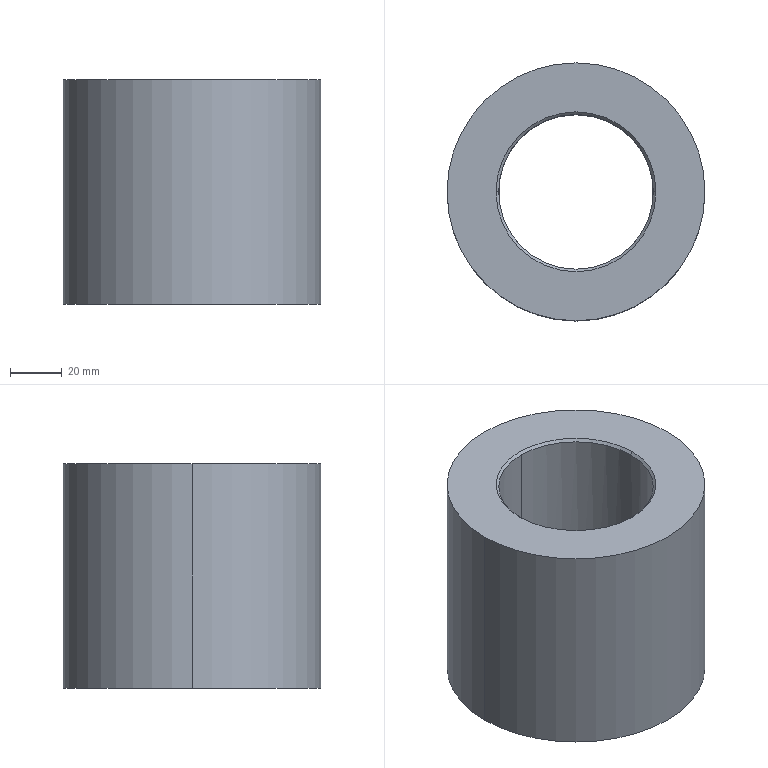Part | SolidWorks | features BaseBody 1 | 1 solid | 8 faces | box 100 x 100 x 87 mm | volume 437214 mm3 | cylinder 4 | cone 2 | plane 2 | commonest cylinder face diameters 60 x2 100 x2
STEP:
#1=CARTESIAN_POINT('',(-30.,0.,41.));
#2=VERTEX_POINT('',#1);
#3=CARTESIAN_POINT('',(0.,-30.,41.));
#4=VERTEX_POINT('',#3);
#5=CARTESIAN_POINT('',(0.,0.,41.));
#6=DIRECTION('',(0.,0.,1.));
#7=DIRECTION('',(-1.,0.,0.));
#8=AXIS2_PLACEMENT_3D('',#5,#6,#7);
#9=CIRCLE('',#8,30.);
#10=EDGE_CURVE('',#2,#4,#9,.T.);
#11=ORIENTED_EDGE('',*,*,#10,.F.);
#12=CARTESIAN_POINT('',(-31.,0.,42.));
#13=VERTEX_POINT('',#12);
#14=CARTESIAN_POINT('',(-31.,0.,42.));
#15=DIRECTION('',(-0.7071,0.,0.7071));
#16=VECTOR('',#15,1000.);
#17=LINE('',#14,#16);
#18=EDGE_CURVE('',#2,#13,#17,.T.);
#19=ORIENTED_EDGE('',*,*,#18,.T.);
#20=CARTESIAN_POINT('',(31.,0.,42.));
#21=VERTEX_POINT('',#20);
#22=CARTESIAN_POINT('',(0.,0.,42.));
#23=DIRECTION('',(0.,0.,-1.));
#24=DIRECTION('',(-1.,0.,0.));
#25=AXIS2_PLACEMENT_3D('',#22,#23,#24);
#26=CIRCLE('',#25,31.);
#27=EDGE_CURVE('',#21,#13,#26,.T.);
#28=ORIENTED_EDGE('',*,*,#27,.F.);
#29=CARTESIAN_POINT('',(30.,0.,41.));
#30=VERTEX_POINT('',#29);
#31=CARTESIAN_POINT('',(31.,0.,42.));
#32=DIRECTION('',(0.7071,0.,0.7071));
#33=VECTOR('',#32,1000.);
#34=LINE('',#31,#33);
#35=EDGE_CURVE('',#30,#21,#34,.T.);
#36=ORIENTED_EDGE('',*,*,#35,.F.);
#37=CARTESIAN_POINT('',(0.,0.,41.));
#38=DIRECTION('',(0.,0.,1.));
#39=DIRECTION('',(-1.,0.,0.));
#40=AXIS2_PLACEMENT_3D('',#37,#38,#39);
#41=CIRCLE('',#40,30.);
#42=EDGE_CURVE('',#4,#30,#41,.T.);
#43=ORIENTED_EDGE('',*,*,#42,.F.);
#44=EDGE_LOOP('',(#11,#19,#28,#36,#43));
#45=FACE_OUTER_BOUND('',#44,.T.);
#46=CARTESIAN_POINT('',(0.,0.,42.));
#47=DIRECTION('',(0.,0.,1.));
#48=DIRECTION('',(1.,0.,0.));
#49=AXIS2_PLACEMENT_3D('',#46,#47,#48);
#50=CONICAL_SURFACE('',#49,31.,0.7854);
#51=ADVANCED_FACE('',(#45),#50,.F.);
#52=ORIENTED_EDGE('',*,*,#42,.T.);
#53=CARTESIAN_POINT('',(0.,30.,41.));
#54=VERTEX_POINT('',#53);
#55=CARTESIAN_POINT('',(0.,0.,41.));
#56=DIRECTION('',(0.,0.,1.));
#57=DIRECTION('',(-1.,0.,0.));
#58=AXIS2_PLACEMENT_3D('',#55,#56,#57);
#59=CIRCLE('',#58,30.);
#60=EDGE_CURVE('',#30,#54,#59,.T.);
#61=ORIENTED_EDGE('',*,*,#60,.T.);
#62=CARTESIAN_POINT('',(0.,30.,-45.));
#63=VERTEX_POINT('',#62);
#64=CARTESIAN_POINT('',(0.,30.,47.));
#65=DIRECTION('',(0.,0.,-1.));
#66=VECTOR('',#65,1000.);
#67=LINE('',#64,#66);
#68=EDGE_CURVE('',#54,#63,#67,.T.);
#69=ORIENTED_EDGE('',*,*,#68,.T.);
#70=CARTESIAN_POINT('',(0.,-30.,-45.));
#71=VERTEX_POINT('',#70);
#72=CARTESIAN_POINT('',(0.,0.,-45.));
#73=DIRECTION('',(0.,0.,1.));
#74=DIRECTION('',(1.,0.,0.));
#75=AXIS2_PLACEMENT_3D('',#72,#73,#74);
#76=CIRCLE('',#75,30.);
#77=EDGE_CURVE('',#71,#63,#76,.T.);
#78=ORIENTED_EDGE('',*,*,#77,.F.);
#79=CARTESIAN_POINT('',(0.,-30.,47.));
#80=DIRECTION('',(0.,0.,-1.));
#81=VECTOR('',#80,1000.);
#82=LINE('',#79,#81);
#83=EDGE_CURVE('',#4,#71,#82,.T.);
#84=ORIENTED_EDGE('',*,*,#83,.F.);
#85=EDGE_LOOP('',(#52,#61,#69,#78,#84));
#86=FACE_OUTER_BOUND('',#85,.T.);
#87=CARTESIAN_POINT('',(0.,0.,47.));
#88=DIRECTION('',(0.,0.,-1.));
#89=DIRECTION('',(0.,-1.,0.));
#90=AXIS2_PLACEMENT_3D('',#87,#88,#89);
#91=CYLINDRICAL_SURFACE('',#90,30.);
#92=ADVANCED_FACE('',(#86),#91,.F.);
#93=CARTESIAN_POINT('',(-50.,0.,42.));
#94=VERTEX_POINT('',#93);
#95=CARTESIAN_POINT('',(50.,0.,42.));
#96=VERTEX_POINT('',#95);
#97=CARTESIAN_POINT('',(0.,0.,42.));
#98=DIRECTION('',(0.,0.,-1.));
#99=DIRECTION('',(-1.,0.,0.));
#100=AXIS2_PLACEMENT_3D('',#97,#98,#99);
#101=CIRCLE('',#100,50.);
#102=EDGE_CURVE('',#94,#96,#101,.T.);
#103=ORIENTED_EDGE('',*,*,#102,.T.);
#104=CARTESIAN_POINT('',(50.,0.,-45.));
#105=VERTEX_POINT('',#104);
#106=CARTESIAN_POINT('',(50.,0.,45.));
#107=DIRECTION('',(0.,0.,-1.));
#108=VECTOR('',#107,1000.);
#109=LINE('',#106,#108);
#110=EDGE_CURVE('',#96,#105,#109,.T.);
#111=ORIENTED_EDGE('',*,*,#110,.T.);
#112=CARTESIAN_POINT('',(-50.,0.,-45.));
#113=VERTEX_POINT('',#112);
#114=CARTESIAN_POINT('',(0.,0.,-45.));
#115=DIRECTION('',(0.,0.,1.));
#116=DIRECTION('',(1.,0.,0.));
#117=AXIS2_PLACEMENT_3D('',#114,#115,#116);
#118=CIRCLE('',#117,50.);
#119=EDGE_CURVE('',#105,#113,#118,.T.);
#120=ORIENTED_EDGE('',*,*,#119,.T.);
#121=CARTESIAN_POINT('',(-50.,0.,45.));
#122=DIRECTION('',(0.,0.,-1.));
#123=VECTOR('',#122,1000.);
#124=LINE('',#121,#123);
#125=EDGE_CURVE('',#94,#113,#124,.T.);
#126=ORIENTED_EDGE('',*,*,#125,.F.);
#127=EDGE_LOOP('',(#103,#111,#120,#126));
#128=FACE_OUTER_BOUND('',#127,.T.);
#129=CARTESIAN_POINT('',(0.,0.,45.));
#130=DIRECTION('',(0.,0.,-1.));
#131=DIRECTION('',(-1.,0.,0.));
#132=AXIS2_PLACEMENT_3D('',#129,#130,#131);
#133=CYLINDRICAL_SURFACE('',#132,50.);
#134=ADVANCED_FACE('',(#128),#133,.T.);
#135=ORIENTED_EDGE('',*,*,#77,.T.);
#136=CARTESIAN_POINT('',(0.,0.,-45.));
#137=DIRECTION('',(0.,0.,1.));
#138=DIRECTION('',(1.,0.,0.));
#139=AXIS2_PLACEMENT_3D('',#136,#137,#138);
#140=CIRCLE('',#139,30.);
#141=EDGE_CURVE('',#63,#71,#140,.T.);
#142=ORIENTED_EDGE('',*,*,#141,.T.);
#143=EDGE_LOOP('',(#135,#142));
#144=FACE_BOUND('',#143,.T.);
#145=CARTESIAN_POINT('',(0.,0.,-45.));
#146=DIRECTION('',(0.,0.,1.));
#147=DIRECTION('',(1.,0.,0.));
#148=AXIS2_PLACEMENT_3D('',#145,#146,#147);
#149=CIRCLE('',#148,50.);
#150=EDGE_CURVE('',#113,#105,#149,.T.);
#151=ORIENTED_EDGE('',*,*,#150,.F.);
#152=ORIENTED_EDGE('',*,*,#119,.F.);
#153=EDGE_LOOP('',(#151,#152));
#154=FACE_OUTER_BOUND('',#153,.T.);
#155=CARTESIAN_POINT('',(0.,0.,-45.));
#156=DIRECTION('',(0.,0.,1.));
#157=DIRECTION('',(1.,0.,0.));
#158=AXIS2_PLACEMENT_3D('',#155,#156,#157);
#159=PLANE('',#158);
#160=ADVANCED_FACE('',(#144,#154),#159,.F.);
#161=ORIENTED_EDGE('',*,*,#110,.F.);
#162=CARTESIAN_POINT('',(0.,0.,42.));
#163=DIRECTION('',(0.,0.,-1.));
#164=DIRECTION('',(-1.,0.,0.));
#165=AXIS2_PLACEMENT_3D('',#162,#163,#164);
#166=CIRCLE('',#165,50.);
#167=EDGE_CURVE('',#96,#94,#166,.T.);
#168=ORIENTED_EDGE('',*,*,#167,.T.);
#169=ORIENTED_EDGE('',*,*,#125,.T.);
#170=ORIENTED_EDGE('',*,*,#150,.T.);
#171=EDGE_LOOP('',(#161,#168,#169,#170));
#172=FACE_OUTER_BOUND('',#171,.T.);
#173=CARTESIAN_POINT('',(0.,0.,45.));
#174=DIRECTION('',(0.,0.,-1.));
#175=DIRECTION('',(-1.,0.,0.));
#176=AXIS2_PLACEMENT_3D('',#173,#174,#175);
#177=CYLINDRICAL_SURFACE('',#176,50.);
#178=ADVANCED_FACE('',(#172),#177,.T.);
#179=ORIENTED_EDGE('',*,*,#27,.T.);
#180=CARTESIAN_POINT('',(0.,0.,42.));
#181=DIRECTION('',(0.,0.,-1.));
#182=DIRECTION('',(-1.,0.,0.));
#183=AXIS2_PLACEMENT_3D('',#180,#181,#182);
#184=CIRCLE('',#183,31.);
#185=EDGE_CURVE('',#13,#21,#184,.T.);
#186=ORIENTED_EDGE('',*,*,#185,.T.);
#187=EDGE_LOOP('',(#179,#186));
#188=FACE_BOUND('',#187,.T.);
#189=ORIENTED_EDGE('',*,*,#102,.F.);
#190=ORIENTED_EDGE('',*,*,#167,.F.);
#191=EDGE_LOOP('',(#189,#190));
#192=FACE_OUTER_BOUND('',#191,.T.);
#193=CARTESIAN_POINT('',(-685.,0.,42.));
#194=DIRECTION('',(0.,0.,-1.));
#195=DIRECTION('',(0.,-1.,0.));
#196=AXIS2_PLACEMENT_3D('',#193,#194,#195);
#197=PLANE('',#196);
#198=ADVANCED_FACE('',(#188,#192),#197,.F.);
#199=ORIENTED_EDGE('',*,*,#68,.F.);
#200=CARTESIAN_POINT('',(0.,0.,41.));
#201=DIRECTION('',(0.,0.,1.));
#202=DIRECTION('',(-1.,0.,0.));
#203=AXIS2_PLACEMENT_3D('',#200,#201,#202);
#204=CIRCLE('',#203,30.);
#205=EDGE_CURVE('',#54,#2,#204,.T.);
#206=ORIENTED_EDGE('',*,*,#205,.T.);
#207=ORIENTED_EDGE('',*,*,#10,.T.);
#208=ORIENTED_EDGE('',*,*,#83,.T.);
#209=ORIENTED_EDGE('',*,*,#141,.F.);
#210=EDGE_LOOP('',(#199,#206,#207,#208,#209));
#211=FACE_OUTER_BOUND('',#210,.T.);
#212=CARTESIAN_POINT('',(0.,0.,47.));
#213=DIRECTION('',(0.,0.,-1.));
#214=DIRECTION('',(0.,-1.,0.));
#215=AXIS2_PLACEMENT_3D('',#212,#213,#214);
#216=CYLINDRICAL_SURFACE('',#215,30.);
#217=ADVANCED_FACE('',(#211),#216,.F.);
#218=ORIENTED_EDGE('',*,*,#18,.F.);
#219=ORIENTED_EDGE('',*,*,#205,.F.);
#220=ORIENTED_EDGE('',*,*,#60,.F.);
#221=ORIENTED_EDGE('',*,*,#35,.T.);
#222=ORIENTED_EDGE('',*,*,#185,.F.);
#223=EDGE_LOOP('',(#218,#219,#220,#221,#222));
#224=FACE_OUTER_BOUND('',#223,.T.);
#225=CARTESIAN_POINT('',(0.,0.,42.));
#226=DIRECTION('',(0.,0.,1.));
#227=DIRECTION('',(1.,0.,0.));
#228=AXIS2_PLACEMENT_3D('',#225,#226,#227);
#229=CONICAL_SURFACE('',#228,31.,0.7854);
#230=ADVANCED_FACE('',(#224),#229,.F.);
#231=CLOSED_SHELL('',(#51,#92,#134,#160,#178,#198,#217,#230));
#232=MANIFOLD_SOLID_BREP('',#231);
#233=CARTESIAN_POINT('',(0.,0.,0.));
#234=DIRECTION('',(0.,0.,1.));
#235=DIRECTION('',(1.,0.,0.));
#236=AXIS2_PLACEMENT_3D('',#233,#234,#235);
#237=(LENGTH_UNIT()NAMED_UNIT(*)SI_UNIT(.MILLI.,.METRE.));
#238=UNCERTAINTY_MEASURE_WITH_UNIT(LENGTH_MEASURE(0.00001),#237,'','');
#239=(NAMED_UNIT(*)PLANE_ANGLE_UNIT()SI_UNIT($,.RADIAN.));
#240=(NAMED_UNIT(*)SI_UNIT($,.STERADIAN.)SOLID_ANGLE_UNIT());
#241=(GEOMETRIC_REPRESENTATION_CONTEXT(3)GLOBAL_UNCERTAINTY_ASSIGNED_CONTEXT((#238))GLOBAL_UNIT_ASSIGNED_CONTEXT((#237,#239,#240))REPRESENTATION_CONTEXT('',''));
#242=ADVANCED_BREP_SHAPE_REPRESENTATION('',(#232,#236),#241);